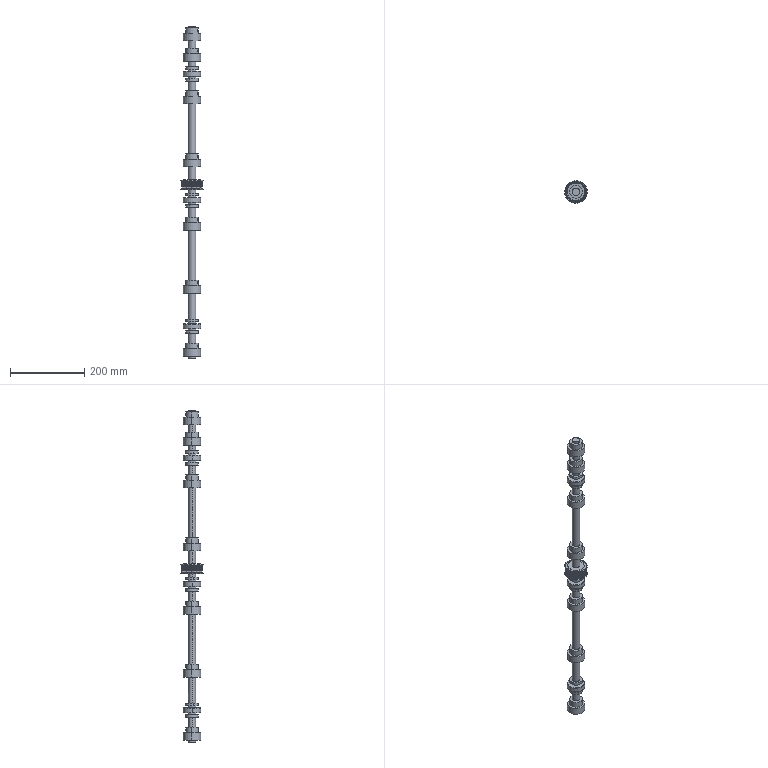Part | SolidWorks | 20 solids | 663 faces | box 61 x 61 x 895 mm | volume 682721 mm3 | cylinder 414 | plane 199 | cone 38 | torus 12 | commonest cylinder face diameters 0.8 x91 1.2 x90 52.85 x39 20 x36 56.45 x36 5 x28